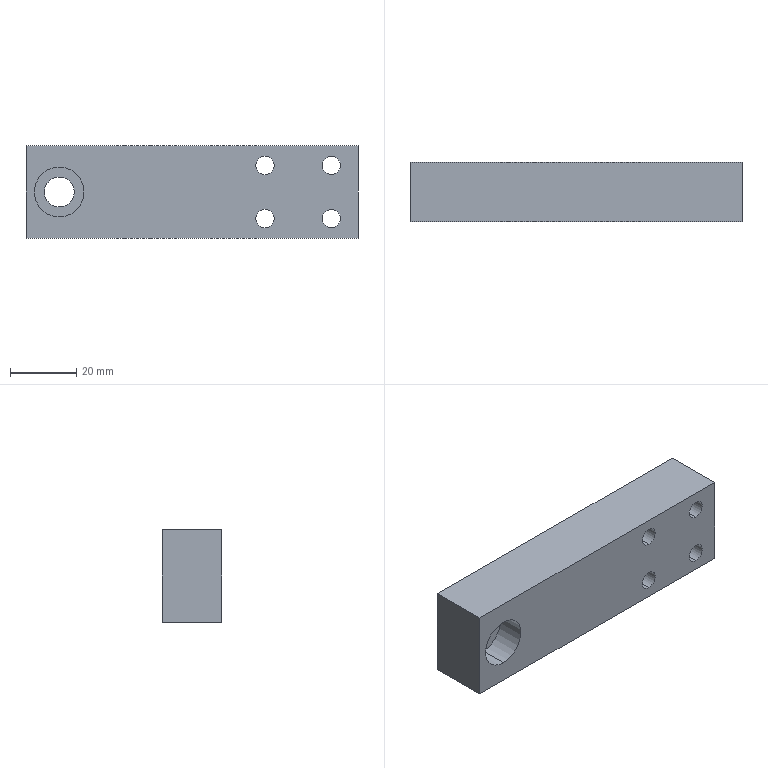Part | STEP file | 1 solid | 31 faces | box 100 x 18 x 28 mm | volume 45388 mm3 | cylinder 20 | plane 11 | commonest cylinder face diameters 5.5 x8 10 x8 9 x2 15 x2